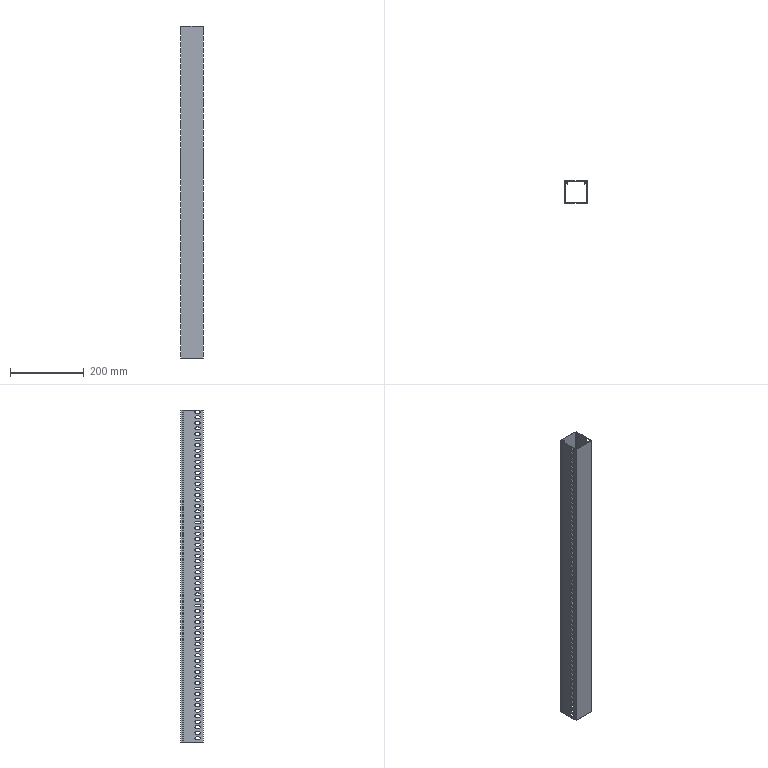Part | SolidWorks | features BaseBody 1 | 1 solid | 506 faces | box 60 x 60 x 900 mm | volume 218608 mm3 | plane 266 | cylinder 240 | commonest cylinder face diameters 8 x240